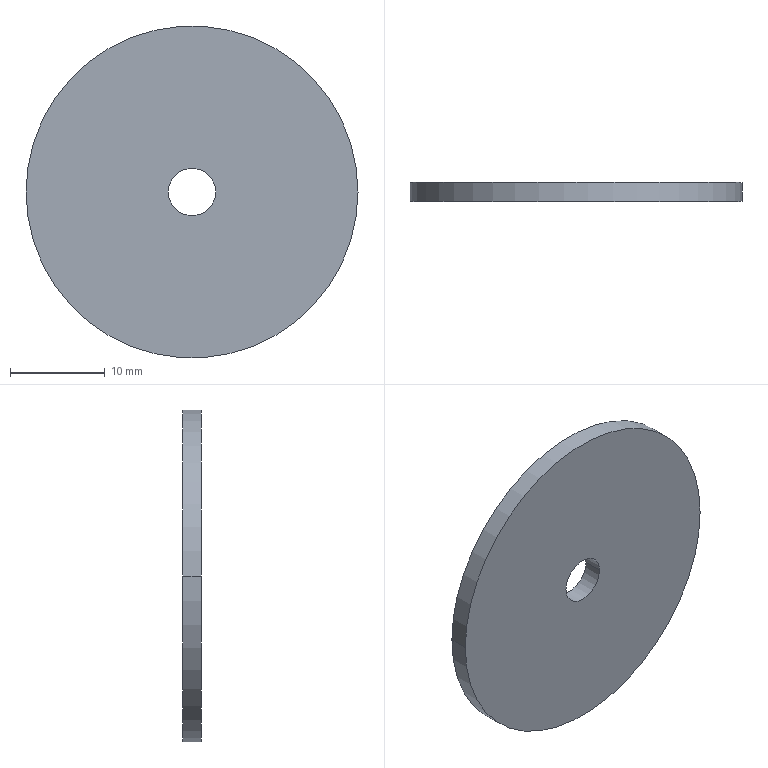Part | STEP file | BAR_INSUL_35 | 1 solid | 6 faces | box 35 x 2 x 35 mm | volume 1885 mm3 | cylinder 4 | plane 2 | commonest cylinder face diameters 5 x2 35 x2
STEP:
#1=CARTESIAN_POINT('',(0.,0.,0.));
#2=DIRECTION('',(0.,0.,1.));
#3=DIRECTION('',(1.,0.,0.));
#4=AXIS2_PLACEMENT_3D('',#1,#2,#3);
#5=CARTESIAN_POINT('',(-17.5,0.,0.));
#6=VERTEX_POINT('',#5);
#7=CARTESIAN_POINT('',(17.5,0.,0.));
#8=VERTEX_POINT('',#7);
#9=CARTESIAN_POINT('',(0.,0.,0.));
#10=DIRECTION('',(0.,1.,0.));
#11=DIRECTION('',(-1.,0.,0.));
#12=AXIS2_PLACEMENT_3D('',#9,#10,#11);
#13=CIRCLE('',#12,17.5);
#14=CARTESIAN_POINT('',(0.,0.,0.));
#15=DIRECTION('',(0.,1.,0.));
#16=DIRECTION('',(-1.,0.,0.));
#17=AXIS2_PLACEMENT_3D('',#14,#15,#16);
#18=PLANE('',#17);
#19=CARTESIAN_POINT('',(0.,0.));
#20=DIRECTION('',(1.,0.));
#21=AXIS2_PLACEMENT_2D('',#19,#20);
#22=CIRCLE('',#21,17.5);
#23=(GEOMETRIC_REPRESENTATION_CONTEXT(2)PARAMETRIC_REPRESENTATION_CONTEXT()REPRESENTATION_CONTEXT('',''));
#24=DEFINITIONAL_REPRESENTATION('',(#22),#23);
#25=PCURVE('',#18,#24);
#26=CARTESIAN_POINT('',(0.,0.,0.));
#27=DIRECTION('',(0.,1.,0.));
#28=DIRECTION('',(-1.,0.,0.));
#29=AXIS2_PLACEMENT_3D('',#26,#27,#28);
#30=CYLINDRICAL_SURFACE('',#29,17.5);
#31=CARTESIAN_POINT('',(0.,0.));
#32=DIRECTION('',(1.,0.));
#33=VECTOR('',#32,1.);
#34=LINE('',#31,#33);
#35=(GEOMETRIC_REPRESENTATION_CONTEXT(2)PARAMETRIC_REPRESENTATION_CONTEXT()REPRESENTATION_CONTEXT('',''));
#36=DEFINITIONAL_REPRESENTATION('',(#34),#35);
#37=PCURVE('',#30,#36);
#38=SURFACE_CURVE('',#13,(#25,#37),.PCURVE_S1.);
#39=EDGE_CURVE('',#6,#8,#38,.T.);
#40=ORIENTED_EDGE('',*,*,#39,.T.);
#41=CARTESIAN_POINT('',(0.,0.,0.));
#42=DIRECTION('',(0.,1.,0.));
#43=DIRECTION('',(1.,0.,0.));
#44=AXIS2_PLACEMENT_3D('',#41,#42,#43);
#45=CIRCLE('',#44,17.5);
#46=CARTESIAN_POINT('',(0.,0.));
#47=DIRECTION('',(-1.,0.));
#48=AXIS2_PLACEMENT_2D('',#46,#47);
#49=CIRCLE('',#48,17.5);
#50=(GEOMETRIC_REPRESENTATION_CONTEXT(2)PARAMETRIC_REPRESENTATION_CONTEXT()REPRESENTATION_CONTEXT('',''));
#51=DEFINITIONAL_REPRESENTATION('',(#49),#50);
#52=PCURVE('',#18,#51);
#53=CARTESIAN_POINT('',(0.,0.,0.));
#54=DIRECTION('',(0.,1.,0.));
#55=DIRECTION('',(-1.,0.,0.));
#56=AXIS2_PLACEMENT_3D('',#53,#54,#55);
#57=CYLINDRICAL_SURFACE('',#56,17.5);
#58=CARTESIAN_POINT('',(3.142,0.));
#59=DIRECTION('',(1.,0.));
#60=VECTOR('',#59,1.);
#61=LINE('',#58,#60);
#62=(GEOMETRIC_REPRESENTATION_CONTEXT(2)PARAMETRIC_REPRESENTATION_CONTEXT()REPRESENTATION_CONTEXT('',''));
#63=DEFINITIONAL_REPRESENTATION('',(#61),#62);
#64=PCURVE('',#57,#63);
#65=SURFACE_CURVE('',#45,(#52,#64),.PCURVE_S1.);
#66=EDGE_CURVE('',#8,#6,#65,.T.);
#67=ORIENTED_EDGE('',*,*,#66,.T.);
#68=EDGE_LOOP('',(#40,#67));
#69=FACE_BOUND('',#68,.F.);
#70=CARTESIAN_POINT('',(-2.5,0.,0.));
#71=VERTEX_POINT('',#70);
#72=CARTESIAN_POINT('',(2.5,0.,0.));
#73=VERTEX_POINT('',#72);
#74=CARTESIAN_POINT('',(0.,0.,0.));
#75=DIRECTION('',(0.,-1.,0.));
#76=DIRECTION('',(-1.,0.,0.));
#77=AXIS2_PLACEMENT_3D('',#74,#75,#76);
#78=CIRCLE('',#77,2.5);
#79=CARTESIAN_POINT('',(2.5,0.));
#80=CARTESIAN_POINT('',(2.5,-4.33));
#81=CARTESIAN_POINT('',(-1.25,-2.165));
#82=CARTESIAN_POINT('',(-5.,0.));
#83=CARTESIAN_POINT('',(-1.25,2.165));
#84=CARTESIAN_POINT('',(2.5,4.33));
#85=CARTESIAN_POINT('',(2.5,0.));
#86=(BOUNDED_CURVE()B_SPLINE_CURVE(2,(#79,#80,#81,#82,#83,#84,#85),.UNSPECIFIED.,.T.,.F.)B_SPLINE_CURVE_WITH_KNOTS((1,2,2,2,2,1),(-2.094,0.,2.094,4.189,6.283,8.378),.UNSPECIFIED.)CURVE()GEOMETRIC_REPRESENTATION_ITEM()RATIONAL_B_SPLINE_CURVE((1.,0.5,1.,0.5,1.,0.5,1.))REPRESENTATION_ITEM(''));
#87=(GEOMETRIC_REPRESENTATION_CONTEXT(2)PARAMETRIC_REPRESENTATION_CONTEXT()REPRESENTATION_CONTEXT('',''));
#88=DEFINITIONAL_REPRESENTATION('',(#86),#87);
#89=PCURVE('',#18,#88);
#90=CARTESIAN_POINT('',(0.,0.,0.));
#91=DIRECTION('',(0.,1.,0.));
#92=DIRECTION('',(-1.,0.,0.));
#93=AXIS2_PLACEMENT_3D('',#90,#91,#92);
#94=CYLINDRICAL_SURFACE('',#93,2.5);
#95=CARTESIAN_POINT('',(6.283,0.));
#96=DIRECTION('',(-1.,0.));
#97=VECTOR('',#96,1.);
#98=LINE('',#95,#97);
#99=(GEOMETRIC_REPRESENTATION_CONTEXT(2)PARAMETRIC_REPRESENTATION_CONTEXT()REPRESENTATION_CONTEXT('',''));
#100=DEFINITIONAL_REPRESENTATION('',(#98),#99);
#101=PCURVE('',#94,#100);
#102=SURFACE_CURVE('',#78,(#89,#101),.PCURVE_S1.);
#103=EDGE_CURVE('',#71,#73,#102,.T.);
#104=ORIENTED_EDGE('',*,*,#103,.T.);
#105=CARTESIAN_POINT('',(0.,0.,0.));
#106=DIRECTION('',(0.,-1.,0.));
#107=DIRECTION('',(1.,0.,0.));
#108=AXIS2_PLACEMENT_3D('',#105,#106,#107);
#109=CIRCLE('',#108,2.5);
#110=CARTESIAN_POINT('',(-2.5,0.));
#111=CARTESIAN_POINT('',(-2.5,4.33));
#112=CARTESIAN_POINT('',(1.25,2.165));
#113=CARTESIAN_POINT('',(5.,0.));
#114=CARTESIAN_POINT('',(1.25,-2.165));
#115=CARTESIAN_POINT('',(-2.5,-4.33));
#116=CARTESIAN_POINT('',(-2.5,0.));
#117=(BOUNDED_CURVE()B_SPLINE_CURVE(2,(#110,#111,#112,#113,#114,#115,#116),.UNSPECIFIED.,.T.,.F.)B_SPLINE_CURVE_WITH_KNOTS((1,2,2,2,2,1),(-2.094,0.,2.094,4.189,6.283,8.378),.UNSPECIFIED.)CURVE()GEOMETRIC_REPRESENTATION_ITEM()RATIONAL_B_SPLINE_CURVE((1.,0.5,1.,0.5,1.,0.5,1.))REPRESENTATION_ITEM(''));
#118=(GEOMETRIC_REPRESENTATION_CONTEXT(2)PARAMETRIC_REPRESENTATION_CONTEXT()REPRESENTATION_CONTEXT('',''));
#119=DEFINITIONAL_REPRESENTATION('',(#117),#118);
#120=PCURVE('',#18,#119);
#121=CARTESIAN_POINT('',(0.,0.,0.));
#122=DIRECTION('',(0.,1.,0.));
#123=DIRECTION('',(-1.,0.,0.));
#124=AXIS2_PLACEMENT_3D('',#121,#122,#123);
#125=CYLINDRICAL_SURFACE('',#124,2.5);
#126=CARTESIAN_POINT('',(3.142,0.));
#127=DIRECTION('',(-1.,0.));
#128=VECTOR('',#127,1.);
#129=LINE('',#126,#128);
#130=(GEOMETRIC_REPRESENTATION_CONTEXT(2)PARAMETRIC_REPRESENTATION_CONTEXT()REPRESENTATION_CONTEXT('',''));
#131=DEFINITIONAL_REPRESENTATION('',(#129),#130);
#132=PCURVE('',#125,#131);
#133=SURFACE_CURVE('',#109,(#120,#132),.PCURVE_S1.);
#134=EDGE_CURVE('',#73,#71,#133,.T.);
#135=ORIENTED_EDGE('',*,*,#134,.T.);
#136=EDGE_LOOP('',(#104,#135));
#137=FACE_BOUND('',#136,.F.);
#138=ADVANCED_FACE('',(#69,#137),#18,.F.);
#139=CARTESIAN_POINT('',(17.5,2.,0.));
#140=VERTEX_POINT('',#139);
#141=CARTESIAN_POINT('',(17.5,0.,0.));
#142=DIRECTION('',(0.,1.,0.));
#143=VECTOR('',#142,1.);
#144=LINE('',#141,#143);
#145=CARTESIAN_POINT('',(3.142,0.));
#146=DIRECTION('',(0.,1.));
#147=VECTOR('',#146,1.);
#148=LINE('',#145,#147);
#149=(GEOMETRIC_REPRESENTATION_CONTEXT(2)PARAMETRIC_REPRESENTATION_CONTEXT()REPRESENTATION_CONTEXT('',''));
#150=DEFINITIONAL_REPRESENTATION('',(#148),#149);
#151=PCURVE('',#30,#150);
#152=CARTESIAN_POINT('',(3.142,0.));
#153=DIRECTION('',(0.,1.));
#154=VECTOR('',#153,1.);
#155=LINE('',#152,#154);
#156=(GEOMETRIC_REPRESENTATION_CONTEXT(2)PARAMETRIC_REPRESENTATION_CONTEXT()REPRESENTATION_CONTEXT('',''));
#157=DEFINITIONAL_REPRESENTATION('',(#155),#156);
#158=PCURVE('',#57,#157);
#159=SURFACE_CURVE('',#144,(#151,#158),.PCURVE_S1.);
#160=EDGE_CURVE('',#8,#140,#159,.T.);
#161=ORIENTED_EDGE('',*,*,#160,.T.);
#162=CARTESIAN_POINT('',(-17.5,2.,0.));
#163=VERTEX_POINT('',#162);
#164=CARTESIAN_POINT('',(0.,2.,0.));
#165=DIRECTION('',(0.,1.,0.));
#166=DIRECTION('',(-1.,0.,0.));
#167=AXIS2_PLACEMENT_3D('',#164,#165,#166);
#168=CIRCLE('',#167,17.5);
#169=CARTESIAN_POINT('',(0.,2.));
#170=DIRECTION('',(1.,0.));
#171=VECTOR('',#170,1.);
#172=LINE('',#169,#171);
#173=(GEOMETRIC_REPRESENTATION_CONTEXT(2)PARAMETRIC_REPRESENTATION_CONTEXT()REPRESENTATION_CONTEXT('',''));
#174=DEFINITIONAL_REPRESENTATION('',(#172),#173);
#175=PCURVE('',#30,#174);
#176=CARTESIAN_POINT('',(0.,2.,0.));
#177=DIRECTION('',(0.,1.,0.));
#178=DIRECTION('',(-1.,0.,0.));
#179=AXIS2_PLACEMENT_3D('',#176,#177,#178);
#180=PLANE('',#179);
#181=CARTESIAN_POINT('',(0.,0.));
#182=DIRECTION('',(1.,0.));
#183=AXIS2_PLACEMENT_2D('',#181,#182);
#184=CIRCLE('',#183,17.5);
#185=(GEOMETRIC_REPRESENTATION_CONTEXT(2)PARAMETRIC_REPRESENTATION_CONTEXT()REPRESENTATION_CONTEXT('',''));
#186=DEFINITIONAL_REPRESENTATION('',(#184),#185);
#187=PCURVE('',#180,#186);
#188=SURFACE_CURVE('',#168,(#175,#187),.PCURVE_S1.);
#189=EDGE_CURVE('',#163,#140,#188,.T.);
#190=ORIENTED_EDGE('',*,*,#189,.F.);
#191=CARTESIAN_POINT('',(-17.5,0.,0.));
#192=DIRECTION('',(0.,1.,0.));
#193=VECTOR('',#192,1.);
#194=LINE('',#191,#193);
#195=CARTESIAN_POINT('',(0.,0.));
#196=DIRECTION('',(0.,1.));
#197=VECTOR('',#196,1.);
#198=LINE('',#195,#197);
#199=(GEOMETRIC_REPRESENTATION_CONTEXT(2)PARAMETRIC_REPRESENTATION_CONTEXT()REPRESENTATION_CONTEXT('',''));
#200=DEFINITIONAL_REPRESENTATION('',(#198),#199);
#201=PCURVE('',#30,#200);
#202=CARTESIAN_POINT('',(6.283,0.));
#203=DIRECTION('',(0.,1.));
#204=VECTOR('',#203,1.);
#205=LINE('',#202,#204);
#206=(GEOMETRIC_REPRESENTATION_CONTEXT(2)PARAMETRIC_REPRESENTATION_CONTEXT()REPRESENTATION_CONTEXT('',''));
#207=DEFINITIONAL_REPRESENTATION('',(#205),#206);
#208=PCURVE('',#57,#207);
#209=SURFACE_CURVE('',#194,(#201,#208),.PCURVE_S1.);
#210=EDGE_CURVE('',#6,#163,#209,.T.);
#211=ORIENTED_EDGE('',*,*,#210,.F.);
#212=ORIENTED_EDGE('',*,*,#39,.T.);
#213=EDGE_LOOP('',(#161,#190,#211,#212));
#214=FACE_BOUND('',#213,.T.);
#215=ADVANCED_FACE('',(#214),#30,.T.);
#216=ORIENTED_EDGE('',*,*,#210,.T.);
#217=CARTESIAN_POINT('',(0.,2.,0.));
#218=DIRECTION('',(0.,1.,0.));
#219=DIRECTION('',(1.,0.,0.));
#220=AXIS2_PLACEMENT_3D('',#217,#218,#219);
#221=CIRCLE('',#220,17.5);
#222=CARTESIAN_POINT('',(3.142,2.));
#223=DIRECTION('',(1.,0.));
#224=VECTOR('',#223,1.);
#225=LINE('',#222,#224);
#226=(GEOMETRIC_REPRESENTATION_CONTEXT(2)PARAMETRIC_REPRESENTATION_CONTEXT()REPRESENTATION_CONTEXT('',''));
#227=DEFINITIONAL_REPRESENTATION('',(#225),#226);
#228=PCURVE('',#57,#227);
#229=CARTESIAN_POINT('',(0.,0.));
#230=DIRECTION('',(-1.,0.));
#231=AXIS2_PLACEMENT_2D('',#229,#230);
#232=CIRCLE('',#231,17.5);
#233=(GEOMETRIC_REPRESENTATION_CONTEXT(2)PARAMETRIC_REPRESENTATION_CONTEXT()REPRESENTATION_CONTEXT('',''));
#234=DEFINITIONAL_REPRESENTATION('',(#232),#233);
#235=PCURVE('',#180,#234);
#236=SURFACE_CURVE('',#221,(#228,#235),.PCURVE_S1.);
#237=EDGE_CURVE('',#140,#163,#236,.T.);
#238=ORIENTED_EDGE('',*,*,#237,.F.);
#239=ORIENTED_EDGE('',*,*,#160,.F.);
#240=ORIENTED_EDGE('',*,*,#66,.T.);
#241=EDGE_LOOP('',(#216,#238,#239,#240));
#242=FACE_BOUND('',#241,.T.);
#243=ADVANCED_FACE('',(#242),#57,.T.);
#244=ORIENTED_EDGE('',*,*,#189,.F.);
#245=ORIENTED_EDGE('',*,*,#237,.F.);
#246=EDGE_LOOP('',(#244,#245));
#247=FACE_BOUND('',#246,.F.);
#248=CARTESIAN_POINT('',(-2.5,2.,0.));
#249=VERTEX_POINT('',#248);
#250=CARTESIAN_POINT('',(2.5,2.,0.));
#251=VERTEX_POINT('',#250);
#252=CARTESIAN_POINT('',(0.,2.,0.));
#253=DIRECTION('',(0.,-1.,0.));
#254=DIRECTION('',(-1.,0.,0.));
#255=AXIS2_PLACEMENT_3D('',#252,#253,#254);
#256=CIRCLE('',#255,2.5);
#257=CARTESIAN_POINT('',(2.5,0.));
#258=CARTESIAN_POINT('',(2.5,-4.33));
#259=CARTESIAN_POINT('',(-1.25,-2.165));
#260=CARTESIAN_POINT('',(-5.,0.));
#261=CARTESIAN_POINT('',(-1.25,2.165));
#262=CARTESIAN_POINT('',(2.5,4.33));
#263=CARTESIAN_POINT('',(2.5,0.));
#264=(BOUNDED_CURVE()B_SPLINE_CURVE(2,(#257,#258,#259,#260,#261,#262,#263),.UNSPECIFIED.,.T.,.F.)B_SPLINE_CURVE_WITH_KNOTS((1,2,2,2,2,1),(-2.094,0.,2.094,4.189,6.283,8.378),.UNSPECIFIED.)CURVE()GEOMETRIC_REPRESENTATION_ITEM()RATIONAL_B_SPLINE_CURVE((1.,0.5,1.,0.5,1.,0.5,1.))REPRESENTATION_ITEM(''));
#265=(GEOMETRIC_REPRESENTATION_CONTEXT(2)PARAMETRIC_REPRESENTATION_CONTEXT()REPRESENTATION_CONTEXT('',''));
#266=DEFINITIONAL_REPRESENTATION('',(#264),#265);
#267=PCURVE('',#180,#266);
#268=CARTESIAN_POINT('',(6.283,2.));
#269=DIRECTION('',(-1.,0.));
#270=VECTOR('',#269,1.);
#271=LINE('',#268,#270);
#272=(GEOMETRIC_REPRESENTATION_CONTEXT(2)PARAMETRIC_REPRESENTATION_CONTEXT()REPRESENTATION_CONTEXT('',''));
#273=DEFINITIONAL_REPRESENTATION('',(#271),#272);
#274=PCURVE('',#94,#273);
#275=SURFACE_CURVE('',#256,(#267,#274),.PCURVE_S1.);
#276=EDGE_CURVE('',#249,#251,#275,.T.);
#277=ORIENTED_EDGE('',*,*,#276,.F.);
#278=CARTESIAN_POINT('',(0.,2.,0.));
#279=DIRECTION('',(0.,-1.,0.));
#280=DIRECTION('',(1.,0.,0.));
#281=AXIS2_PLACEMENT_3D('',#278,#279,#280);
#282=CIRCLE('',#281,2.5);
#283=CARTESIAN_POINT('',(-2.5,0.));
#284=CARTESIAN_POINT('',(-2.5,4.33));
#285=CARTESIAN_POINT('',(1.25,2.165));
#286=CARTESIAN_POINT('',(5.,0.));
#287=CARTESIAN_POINT('',(1.25,-2.165));
#288=CARTESIAN_POINT('',(-2.5,-4.33));
#289=CARTESIAN_POINT('',(-2.5,0.));
#290=(BOUNDED_CURVE()B_SPLINE_CURVE(2,(#283,#284,#285,#286,#287,#288,#289),.UNSPECIFIED.,.T.,.F.)B_SPLINE_CURVE_WITH_KNOTS((1,2,2,2,2,1),(-2.094,0.,2.094,4.189,6.283,8.378),.UNSPECIFIED.)CURVE()GEOMETRIC_REPRESENTATION_ITEM()RATIONAL_B_SPLINE_CURVE((1.,0.5,1.,0.5,1.,0.5,1.))REPRESENTATION_ITEM(''));
#291=(GEOMETRIC_REPRESENTATION_CONTEXT(2)PARAMETRIC_REPRESENTATION_CONTEXT()REPRESENTATION_CONTEXT('',''));
#292=DEFINITIONAL_REPRESENTATION('',(#290),#291);
#293=PCURVE('',#180,#292);
#294=CARTESIAN_POINT('',(3.142,2.));
#295=DIRECTION('',(-1.,0.));
#296=VECTOR('',#295,1.);
#297=LINE('',#294,#296);
#298=(GEOMETRIC_REPRESENTATION_CONTEXT(2)PARAMETRIC_REPRESENTATION_CONTEXT()REPRESENTATION_CONTEXT('',''));
#299=DEFINITIONAL_REPRESENTATION('',(#297),#298);
#300=PCURVE('',#125,#299);
#301=SURFACE_CURVE('',#282,(#293,#300),.PCURVE_S1.);
#302=EDGE_CURVE('',#251,#249,#301,.T.);
#303=ORIENTED_EDGE('',*,*,#302,.F.);
#304=EDGE_LOOP('',(#277,#303));
#305=FACE_BOUND('',#304,.F.);
#306=ADVANCED_FACE('',(#247,#305),#180,.T.);
#307=ORIENTED_EDGE('',*,*,#103,.F.);
#308=CARTESIAN_POINT('',(-2.5,0.,0.));
#309=DIRECTION('',(0.,1.,0.));
#310=VECTOR('',#309,1.);
#311=LINE('',#308,#310);
#312=CARTESIAN_POINT('',(6.283,0.));
#313=DIRECTION('',(0.,1.));
#314=VECTOR('',#313,1.);
#315=LINE('',#312,#314);
#316=(GEOMETRIC_REPRESENTATION_CONTEXT(2)PARAMETRIC_REPRESENTATION_CONTEXT()REPRESENTATION_CONTEXT('',''));
#317=DEFINITIONAL_REPRESENTATION('',(#315),#316);
#318=PCURVE('',#94,#317);
#319=CARTESIAN_POINT('',(0.,0.));
#320=DIRECTION('',(0.,1.));
#321=VECTOR('',#320,1.);
#322=LINE('',#319,#321);
#323=(GEOMETRIC_REPRESENTATION_CONTEXT(2)PARAMETRIC_REPRESENTATION_CONTEXT()REPRESENTATION_CONTEXT('',''));
#324=DEFINITIONAL_REPRESENTATION('',(#322),#323);
#325=PCURVE('',#125,#324);
#326=SURFACE_CURVE('',#311,(#318,#325),.PCURVE_S1.);
#327=EDGE_CURVE('',#71,#249,#326,.T.);
#328=ORIENTED_EDGE('',*,*,#327,.T.);
#329=ORIENTED_EDGE('',*,*,#276,.T.);
#330=CARTESIAN_POINT('',(2.5,0.,0.));
#331=DIRECTION('',(0.,1.,0.));
#332=VECTOR('',#331,1.);
#333=LINE('',#330,#332);
#334=CARTESIAN_POINT('',(3.142,0.));
#335=DIRECTION('',(0.,1.));
#336=VECTOR('',#335,1.);
#337=LINE('',#334,#336);
#338=(GEOMETRIC_REPRESENTATION_CONTEXT(2)PARAMETRIC_REPRESENTATION_CONTEXT()REPRESENTATION_CONTEXT('',''));
#339=DEFINITIONAL_REPRESENTATION('',(#337),#338);
#340=PCURVE('',#94,#339);
#341=CARTESIAN_POINT('',(3.142,0.));
#342=DIRECTION('',(0.,1.));
#343=VECTOR('',#342,1.);
#344=LINE('',#341,#343);
#345=(GEOMETRIC_REPRESENTATION_CONTEXT(2)PARAMETRIC_REPRESENTATION_CONTEXT()REPRESENTATION_CONTEXT('',''));
#346=DEFINITIONAL_REPRESENTATION('',(#344),#345);
#347=PCURVE('',#125,#346);
#348=SURFACE_CURVE('',#333,(#340,#347),.PCURVE_S1.);
#349=EDGE_CURVE('',#73,#251,#348,.T.);
#350=ORIENTED_EDGE('',*,*,#349,.F.);
#351=EDGE_LOOP('',(#307,#328,#329,#350));
#352=FACE_BOUND('',#351,.F.);
#353=ADVANCED_FACE('',(#352),#94,.F.);
#354=ORIENTED_EDGE('',*,*,#134,.F.);
#355=ORIENTED_EDGE('',*,*,#349,.T.);
#356=ORIENTED_EDGE('',*,*,#302,.T.);
#357=ORIENTED_EDGE('',*,*,#327,.F.);
#358=EDGE_LOOP('',(#354,#355,#356,#357));
#359=FACE_BOUND('',#358,.F.);
#360=ADVANCED_FACE('',(#359),#125,.F.);
#361=CLOSED_SHELL('',(#138,#215,#243,#306,#353,#360));
#362=MANIFOLD_SOLID_BREP('',#361);
#363=(LENGTH_UNIT()NAMED_UNIT(*)SI_UNIT(.MILLI.,.METRE.));
#364=UNCERTAINTY_MEASURE_WITH_UNIT(LENGTH_MEASURE(0.0000001),#363,'','');
#365=(NAMED_UNIT(*)PLANE_ANGLE_UNIT()SI_UNIT($,.RADIAN.));
#366=(NAMED_UNIT(*)SI_UNIT($,.STERADIAN.)SOLID_ANGLE_UNIT());
#367=(GEOMETRIC_REPRESENTATION_CONTEXT(3)GLOBAL_UNCERTAINTY_ASSIGNED_CONTEXT((#364))GLOBAL_UNIT_ASSIGNED_CONTEXT((#363,#365,#366))REPRESENTATION_CONTEXT('',''));
#368=ADVANCED_BREP_SHAPE_REPRESENTATION('',(#4,#362),#367);